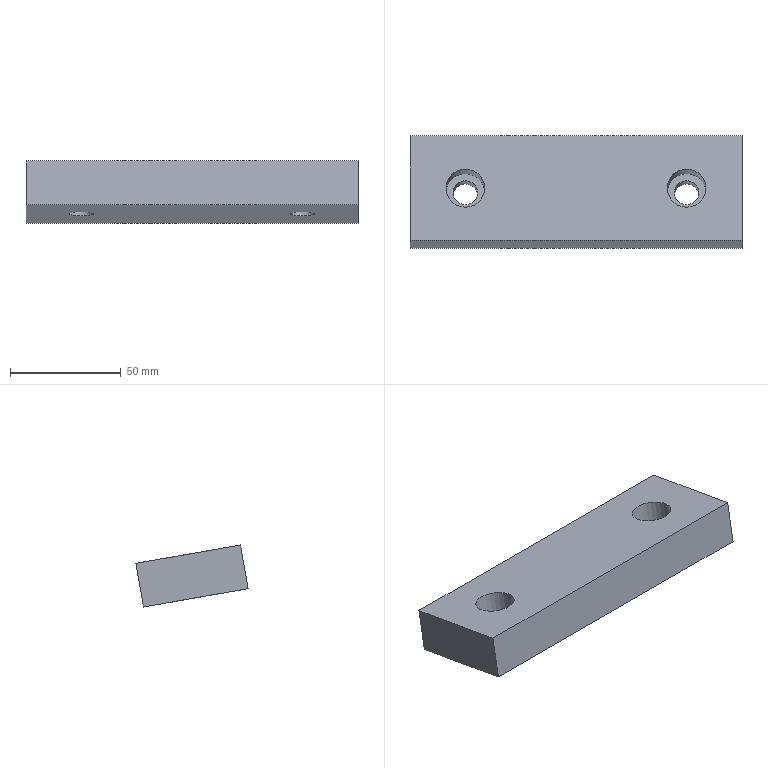Part | NX | features solid 2 | 1 solid | 12 faces | box 150 x 50.744 x 28.031 mm | volume 136707 mm3 | plane 8 | cylinder 4 | commonest cylinder face diameters 11 x2 17.5 x2
STEP:
#1=CARTESIAN_POINT('',(-366.2,-816.957,-253.449));
#2=VERTEX_POINT('',#1);
#3=CARTESIAN_POINT('',(-366.2,-820.43,-273.145));
#4=VERTEX_POINT('',#3);
#5=CARTESIAN_POINT('',(-366.2,-816.957,-253.449));
#6=DIRECTION('',(0.,0.1736,0.9848));
#7=VECTOR('',#6,1000.);
#8=LINE('',#5,#7);
#9=EDGE_CURVE('',#2,#4,#8,.F.);
#10=ORIENTED_EDGE('',*,*,#9,.F.);
#11=CARTESIAN_POINT('',(-366.2,-864.228,-245.114));
#12=VERTEX_POINT('',#11);
#13=CARTESIAN_POINT('',(-366.2,-864.228,-245.114));
#14=DIRECTION('',(0.,0.9848,-0.1736));
#15=VECTOR('',#14,1000.);
#16=LINE('',#13,#15);
#17=EDGE_CURVE('',#12,#2,#16,.T.);
#18=ORIENTED_EDGE('',*,*,#17,.F.);
#19=CARTESIAN_POINT('',(-366.2,-867.701,-264.81));
#20=VERTEX_POINT('',#19);
#21=CARTESIAN_POINT('',(-366.2,-864.228,-245.114));
#22=DIRECTION('',(0.,0.1736,0.9848));
#23=VECTOR('',#22,1000.);
#24=LINE('',#21,#23);
#25=EDGE_CURVE('',#12,#20,#24,.F.);
#26=ORIENTED_EDGE('',*,*,#25,.T.);
#27=CARTESIAN_POINT('',(-366.2,-867.701,-264.81));
#28=DIRECTION('',(0.,0.9848,-0.1736));
#29=VECTOR('',#28,1000.);
#30=LINE('',#27,#29);
#31=EDGE_CURVE('',#20,#4,#30,.T.);
#32=ORIENTED_EDGE('',*,*,#31,.T.);
#33=EDGE_LOOP('',(#10,#18,#26,#32));
#34=FACE_BOUND('',#33,.T.);
#35=CARTESIAN_POINT('',(-366.2,-864.228,-245.114));
#36=DIRECTION('',(-1.,0.,0.));
#37=DIRECTION('',(0.,0.,-1.));
#38=AXIS2_PLACEMENT_3D('',#35,#36,#37);
#39=PLANE('',#38);
#40=ADVANCED_FACE('',(#34),#39,.F.);
#41=CARTESIAN_POINT('',(-491.2,-831.976,-250.801));
#42=VERTEX_POINT('',#41);
#43=CARTESIAN_POINT('',(-491.2,-840.593,-249.281));
#44=DIRECTION('',(0.,0.1736,0.9848));
#45=DIRECTION('',(0.,0.9848,-0.1736));
#46=AXIS2_PLACEMENT_3D('',#43,#44,#45);
#47=CIRCLE('',#46,8.75);
#48=EDGE_CURVE('',#42,#42,#47,.T.);
#49=ORIENTED_EDGE('',*,*,#48,.F.);
#50=EDGE_LOOP('',(#49));
#51=FACE_BOUND('',#50,.T.);
#52=CARTESIAN_POINT('',(-391.2,-831.976,-250.801));
#53=VERTEX_POINT('',#52);
#54=CARTESIAN_POINT('',(-391.2,-840.593,-249.281));
#55=DIRECTION('',(0.,0.1736,0.9848));
#56=DIRECTION('',(0.,0.9848,-0.1736));
#57=AXIS2_PLACEMENT_3D('',#54,#55,#56);
#58=CIRCLE('',#57,8.75);
#59=EDGE_CURVE('',#53,#53,#58,.T.);
#60=ORIENTED_EDGE('',*,*,#59,.F.);
#61=EDGE_LOOP('',(#60));
#62=FACE_BOUND('',#61,.T.);
#63=CARTESIAN_POINT('',(-516.2,-816.957,-253.449));
#64=VERTEX_POINT('',#63);
#65=CARTESIAN_POINT('',(-366.2,-816.957,-253.449));
#66=DIRECTION('',(1.,0.,0.));
#67=VECTOR('',#66,1000.);
#68=LINE('',#65,#67);
#69=EDGE_CURVE('',#2,#64,#68,.F.);
#70=ORIENTED_EDGE('',*,*,#69,.T.);
#71=CARTESIAN_POINT('',(-516.2,-864.228,-245.114));
#72=VERTEX_POINT('',#71);
#73=CARTESIAN_POINT('',(-516.2,-864.228,-245.114));
#74=DIRECTION('',(0.,0.9848,-0.1736));
#75=VECTOR('',#74,1000.);
#76=LINE('',#73,#75);
#77=EDGE_CURVE('',#72,#64,#76,.T.);
#78=ORIENTED_EDGE('',*,*,#77,.F.);
#79=CARTESIAN_POINT('',(-366.2,-864.228,-245.114));
#80=DIRECTION('',(1.,0.,0.));
#81=VECTOR('',#80,1000.);
#82=LINE('',#79,#81);
#83=EDGE_CURVE('',#12,#72,#82,.F.);
#84=ORIENTED_EDGE('',*,*,#83,.F.);
#85=ORIENTED_EDGE('',*,*,#17,.T.);
#86=EDGE_LOOP('',(#70,#78,#84,#85));
#87=FACE_BOUND('',#86,.T.);
#88=CARTESIAN_POINT('',(-366.2,-864.228,-245.114));
#89=DIRECTION('',(0.,0.1736,0.9848));
#90=DIRECTION('',(0.,-0.9848,0.1736));
#91=AXIS2_PLACEMENT_3D('',#88,#89,#90);
#92=PLANE('',#91);
#93=ADVANCED_FACE('',(#51,#62,#87),#92,.T.);
#94=CARTESIAN_POINT('',(-516.2,-820.43,-273.145));
#95=VERTEX_POINT('',#94);
#96=CARTESIAN_POINT('',(-516.2,-816.957,-253.449));
#97=DIRECTION('',(0.,-0.1736,-0.9848));
#98=VECTOR('',#97,1000.);
#99=LINE('',#96,#98);
#100=EDGE_CURVE('',#64,#95,#99,.T.);
#101=ORIENTED_EDGE('',*,*,#100,.T.);
#102=CARTESIAN_POINT('',(-516.2,-867.701,-264.81));
#103=VERTEX_POINT('',#102);
#104=CARTESIAN_POINT('',(-516.2,-867.701,-264.81));
#105=DIRECTION('',(0.,0.9848,-0.1736));
#106=VECTOR('',#105,1000.);
#107=LINE('',#104,#106);
#108=EDGE_CURVE('',#103,#95,#107,.T.);
#109=ORIENTED_EDGE('',*,*,#108,.F.);
#110=CARTESIAN_POINT('',(-516.2,-864.228,-245.114));
#111=DIRECTION('',(0.,-0.1736,-0.9848));
#112=VECTOR('',#111,1000.);
#113=LINE('',#110,#112);
#114=EDGE_CURVE('',#72,#103,#113,.T.);
#115=ORIENTED_EDGE('',*,*,#114,.F.);
#116=ORIENTED_EDGE('',*,*,#77,.T.);
#117=EDGE_LOOP('',(#101,#109,#115,#116));
#118=FACE_BOUND('',#117,.T.);
#119=CARTESIAN_POINT('',(-516.2,-864.228,-245.114));
#120=DIRECTION('',(-1.,0.,0.));
#121=DIRECTION('',(0.,0.,-1.));
#122=AXIS2_PLACEMENT_3D('',#119,#120,#121);
#123=PLANE('',#122);
#124=ADVANCED_FACE('',(#118),#123,.T.);
#125=CARTESIAN_POINT('',(-491.2,-849.482,-268.022));
#126=VERTEX_POINT('',#125);
#127=CARTESIAN_POINT('',(-491.2,-844.066,-268.977));
#128=DIRECTION('',(0.,-0.1736,-0.9848));
#129=DIRECTION('',(0.,-0.9848,0.1736));
#130=AXIS2_PLACEMENT_3D('',#127,#128,#129);
#131=CIRCLE('',#130,5.5);
#132=EDGE_CURVE('',#126,#126,#131,.T.);
#133=ORIENTED_EDGE('',*,*,#132,.F.);
#134=EDGE_LOOP('',(#133));
#135=FACE_BOUND('',#134,.T.);
#136=CARTESIAN_POINT('',(-391.2,-849.482,-268.022));
#137=VERTEX_POINT('',#136);
#138=CARTESIAN_POINT('',(-391.2,-844.066,-268.977));
#139=DIRECTION('',(0.,-0.1736,-0.9848));
#140=DIRECTION('',(0.,-0.9848,0.1736));
#141=AXIS2_PLACEMENT_3D('',#138,#139,#140);
#142=CIRCLE('',#141,5.5);
#143=EDGE_CURVE('',#137,#137,#142,.T.);
#144=ORIENTED_EDGE('',*,*,#143,.F.);
#145=EDGE_LOOP('',(#144));
#146=FACE_BOUND('',#145,.T.);
#147=CARTESIAN_POINT('',(-366.2,-820.43,-273.145));
#148=DIRECTION('',(1.,0.,0.));
#149=VECTOR('',#148,1000.);
#150=LINE('',#147,#149);
#151=EDGE_CURVE('',#4,#95,#150,.F.);
#152=ORIENTED_EDGE('',*,*,#151,.F.);
#153=ORIENTED_EDGE('',*,*,#31,.F.);
#154=CARTESIAN_POINT('',(-366.2,-867.701,-264.81));
#155=DIRECTION('',(1.,0.,0.));
#156=VECTOR('',#155,1000.);
#157=LINE('',#154,#156);
#158=EDGE_CURVE('',#20,#103,#157,.F.);
#159=ORIENTED_EDGE('',*,*,#158,.T.);
#160=ORIENTED_EDGE('',*,*,#108,.T.);
#161=EDGE_LOOP('',(#152,#153,#159,#160));
#162=FACE_BOUND('',#161,.T.);
#163=CARTESIAN_POINT('',(-366.2,-867.701,-264.81));
#164=DIRECTION('',(0.,0.1736,0.9848));
#165=DIRECTION('',(0.,-0.9848,0.1736));
#166=AXIS2_PLACEMENT_3D('',#163,#164,#165);
#167=PLANE('',#166);
#168=ADVANCED_FACE('',(#135,#146,#162),#167,.F.);
#169=ORIENTED_EDGE('',*,*,#25,.F.);
#170=ORIENTED_EDGE('',*,*,#83,.T.);
#171=ORIENTED_EDGE('',*,*,#114,.T.);
#172=ORIENTED_EDGE('',*,*,#158,.F.);
#173=EDGE_LOOP('',(#169,#170,#171,#172));
#174=FACE_BOUND('',#173,.T.);
#175=CARTESIAN_POINT('',(-366.2,-864.228,-245.114));
#176=DIRECTION('',(0.,0.9848,-0.1736));
#177=DIRECTION('',(-1.,0.,0.));
#178=AXIS2_PLACEMENT_3D('',#175,#176,#177);
#179=PLANE('',#178);
#180=ADVANCED_FACE('',(#174),#179,.F.);
#181=ORIENTED_EDGE('',*,*,#9,.T.);
#182=ORIENTED_EDGE('',*,*,#151,.T.);
#183=ORIENTED_EDGE('',*,*,#100,.F.);
#184=ORIENTED_EDGE('',*,*,#69,.F.);
#185=EDGE_LOOP('',(#181,#182,#183,#184));
#186=FACE_BOUND('',#185,.T.);
#187=CARTESIAN_POINT('',(-366.2,-816.957,-253.449));
#188=DIRECTION('',(0.,0.9848,-0.1736));
#189=DIRECTION('',(-1.,0.,0.));
#190=AXIS2_PLACEMENT_3D('',#187,#188,#189);
#191=PLANE('',#190);
#192=ADVANCED_FACE('',(#186),#191,.T.);
#193=CARTESIAN_POINT('',(-391.2,-837.26,-262.054));
#194=VERTEX_POINT('',#193);
#195=CARTESIAN_POINT('',(-391.2,-842.677,-261.099));
#196=DIRECTION('',(0.,0.1736,0.9848));
#197=DIRECTION('',(0.,0.9848,-0.1736));
#198=AXIS2_PLACEMENT_3D('',#195,#196,#197);
#199=CIRCLE('',#198,5.5);
#200=EDGE_CURVE('',#194,#194,#199,.T.);
#201=ORIENTED_EDGE('',*,*,#200,.T.);
#202=EDGE_LOOP('',(#201));
#203=FACE_BOUND('',#202,.T.);
#204=ORIENTED_EDGE('',*,*,#143,.T.);
#205=EDGE_LOOP('',(#204));
#206=FACE_BOUND('',#205,.T.);
#207=CARTESIAN_POINT('',(-391.2,-849.275,-298.522));
#208=DIRECTION('',(0.,-0.1736,-0.9848));
#209=DIRECTION('',(0.,0.9848,-0.1736));
#210=AXIS2_PLACEMENT_3D('',#207,#208,#209);
#211=CYLINDRICAL_SURFACE('',#210,5.5);
#212=ADVANCED_FACE('',(#203,#206),#211,.F.);
#213=ORIENTED_EDGE('',*,*,#200,.F.);
#214=EDGE_LOOP('',(#213));
#215=FACE_BOUND('',#214,.T.);
#216=CARTESIAN_POINT('',(-391.2,-834.059,-262.618));
#217=VERTEX_POINT('',#216);
#218=CARTESIAN_POINT('',(-391.2,-842.677,-261.099));
#219=DIRECTION('',(0.,0.1736,0.9848));
#220=DIRECTION('',(0.,0.9848,-0.1736));
#221=AXIS2_PLACEMENT_3D('',#218,#219,#220);
#222=CIRCLE('',#221,8.75);
#223=EDGE_CURVE('',#217,#217,#222,.T.);
#224=ORIENTED_EDGE('',*,*,#223,.T.);
#225=EDGE_LOOP('',(#224));
#226=FACE_BOUND('',#225,.T.);
#227=CARTESIAN_POINT('',(-391.2,-842.677,-261.099));
#228=DIRECTION('',(0.,-0.1736,-0.9848));
#229=DIRECTION('',(0.,0.9848,-0.1736));
#230=AXIS2_PLACEMENT_3D('',#227,#228,#229);
#231=PLANE('',#230);
#232=ADVANCED_FACE('',(#215,#226),#231,.F.);
#233=ORIENTED_EDGE('',*,*,#223,.F.);
#234=EDGE_LOOP('',(#233));
#235=FACE_BOUND('',#234,.T.);
#236=ORIENTED_EDGE('',*,*,#59,.T.);
#237=EDGE_LOOP('',(#236));
#238=FACE_BOUND('',#237,.T.);
#239=CARTESIAN_POINT('',(-391.2,-840.593,-249.281));
#240=DIRECTION('',(0.,-0.1736,-0.9848));
#241=DIRECTION('',(0.,0.9848,-0.1736));
#242=AXIS2_PLACEMENT_3D('',#239,#240,#241);
#243=CYLINDRICAL_SURFACE('',#242,8.75);
#244=ADVANCED_FACE('',(#235,#238),#243,.F.);
#245=CARTESIAN_POINT('',(-491.2,-837.26,-262.054));
#246=VERTEX_POINT('',#245);
#247=CARTESIAN_POINT('',(-491.2,-842.677,-261.099));
#248=DIRECTION('',(0.,0.1736,0.9848));
#249=DIRECTION('',(0.,0.9848,-0.1736));
#250=AXIS2_PLACEMENT_3D('',#247,#248,#249);
#251=CIRCLE('',#250,5.5);
#252=EDGE_CURVE('',#246,#246,#251,.T.);
#253=ORIENTED_EDGE('',*,*,#252,.T.);
#254=EDGE_LOOP('',(#253));
#255=FACE_BOUND('',#254,.T.);
#256=ORIENTED_EDGE('',*,*,#132,.T.);
#257=EDGE_LOOP('',(#256));
#258=FACE_BOUND('',#257,.T.);
#259=CARTESIAN_POINT('',(-491.2,-849.275,-298.522));
#260=DIRECTION('',(0.,-0.1736,-0.9848));
#261=DIRECTION('',(0.,0.9848,-0.1736));
#262=AXIS2_PLACEMENT_3D('',#259,#260,#261);
#263=CYLINDRICAL_SURFACE('',#262,5.5);
#264=ADVANCED_FACE('',(#255,#258),#263,.F.);
#265=ORIENTED_EDGE('',*,*,#252,.F.);
#266=EDGE_LOOP('',(#265));
#267=FACE_BOUND('',#266,.T.);
#268=CARTESIAN_POINT('',(-491.2,-834.059,-262.618));
#269=VERTEX_POINT('',#268);
#270=CARTESIAN_POINT('',(-491.2,-842.677,-261.099));
#271=DIRECTION('',(0.,0.1736,0.9848));
#272=DIRECTION('',(0.,0.9848,-0.1736));
#273=AXIS2_PLACEMENT_3D('',#270,#271,#272);
#274=CIRCLE('',#273,8.75);
#275=EDGE_CURVE('',#269,#269,#274,.T.);
#276=ORIENTED_EDGE('',*,*,#275,.T.);
#277=EDGE_LOOP('',(#276));
#278=FACE_BOUND('',#277,.T.);
#279=CARTESIAN_POINT('',(-491.2,-842.677,-261.099));
#280=DIRECTION('',(0.,-0.1736,-0.9848));
#281=DIRECTION('',(0.,0.9848,-0.1736));
#282=AXIS2_PLACEMENT_3D('',#279,#280,#281);
#283=PLANE('',#282);
#284=ADVANCED_FACE('',(#267,#278),#283,.F.);
#285=ORIENTED_EDGE('',*,*,#275,.F.);
#286=EDGE_LOOP('',(#285));
#287=FACE_BOUND('',#286,.T.);
#288=ORIENTED_EDGE('',*,*,#48,.T.);
#289=EDGE_LOOP('',(#288));
#290=FACE_BOUND('',#289,.T.);
#291=CARTESIAN_POINT('',(-491.2,-840.593,-249.281));
#292=DIRECTION('',(0.,-0.1736,-0.9848));
#293=DIRECTION('',(0.,0.9848,-0.1736));
#294=AXIS2_PLACEMENT_3D('',#291,#292,#293);
#295=CYLINDRICAL_SURFACE('',#294,8.75);
#296=ADVANCED_FACE('',(#287,#290),#295,.F.);
#297=CLOSED_SHELL('',(#40,#93,#124,#168,#180,#192,#212,#232,#244,#264,#284,#296));
#298=MANIFOLD_SOLID_BREP('',#297);
#299=(LENGTH_UNIT()NAMED_UNIT(*)SI_UNIT(.MILLI.,.METRE.));
#300=UNCERTAINTY_MEASURE_WITH_UNIT(LENGTH_MEASURE(0.00001),#299,'','');
#301=(NAMED_UNIT(*)PLANE_ANGLE_UNIT()SI_UNIT($,.RADIAN.));
#302=(NAMED_UNIT(*)SI_UNIT($,.STERADIAN.)SOLID_ANGLE_UNIT());
#303=(GEOMETRIC_REPRESENTATION_CONTEXT(3)GLOBAL_UNCERTAINTY_ASSIGNED_CONTEXT((#300))GLOBAL_UNIT_ASSIGNED_CONTEXT((#299,#301,#302))REPRESENTATION_CONTEXT('',''));
#304=ADVANCED_BREP_SHAPE_REPRESENTATION('',(#298),#303);